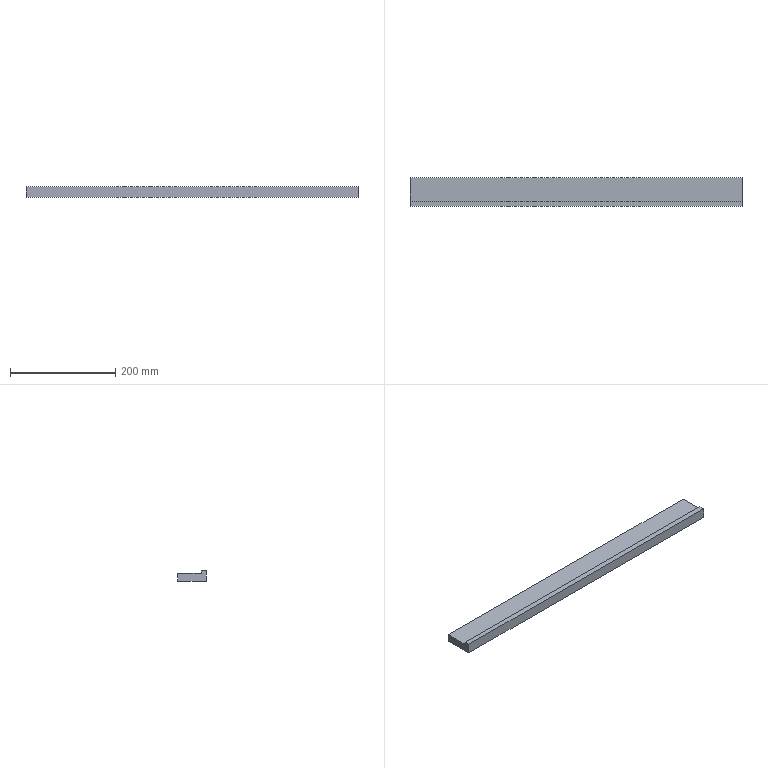Part | SolidWorks | features Extrusion 1 | 1 solid | 8 faces | box 630 x 55 x 20 mm | volume 551250 mm3 | plane 8
STEP:
#1=CARTESIAN_POINT('',(0.,48.109,31.215));
#2=VERTEX_POINT('',#1);
#3=CARTESIAN_POINT('',(0.,48.109,46.215));
#4=VERTEX_POINT('',#3);
#5=CARTESIAN_POINT('',(0.,48.109,31.215));
#6=DIRECTION('',(0.,0.,1.));
#7=VECTOR('',#6,1000.);
#8=LINE('',#5,#7);
#9=EDGE_CURVE('',#2,#4,#8,.T.);
#10=ORIENTED_EDGE('',*,*,#9,.F.);
#11=CARTESIAN_POINT('',(-630.,48.109,31.215));
#12=VERTEX_POINT('',#11);
#13=CARTESIAN_POINT('',(-630.,48.109,31.215));
#14=DIRECTION('',(1.,0.,0.));
#15=VECTOR('',#14,1000.);
#16=LINE('',#13,#15);
#17=EDGE_CURVE('',#12,#2,#16,.T.);
#18=ORIENTED_EDGE('',*,*,#17,.F.);
#19=CARTESIAN_POINT('',(-630.,48.109,46.215));
#20=VERTEX_POINT('',#19);
#21=CARTESIAN_POINT('',(-630.,48.109,31.215));
#22=DIRECTION('',(0.,0.,1.));
#23=VECTOR('',#22,1000.);
#24=LINE('',#21,#23);
#25=EDGE_CURVE('',#12,#20,#24,.T.);
#26=ORIENTED_EDGE('',*,*,#25,.T.);
#27=CARTESIAN_POINT('',(-630.,48.109,46.215));
#28=DIRECTION('',(1.,0.,0.));
#29=VECTOR('',#28,1000.);
#30=LINE('',#27,#29);
#31=EDGE_CURVE('',#20,#4,#30,.T.);
#32=ORIENTED_EDGE('',*,*,#31,.T.);
#33=EDGE_LOOP('',(#10,#18,#26,#32));
#34=FACE_OUTER_BOUND('',#33,.T.);
#35=CARTESIAN_POINT('',(-630.,48.109,31.215));
#36=DIRECTION('',(0.,1.,0.));
#37=DIRECTION('',(0.,0.,1.));
#38=AXIS2_PLACEMENT_3D('',#35,#36,#37);
#39=PLANE('',#38);
#40=ADVANCED_FACE('',(#34),#39,.T.);
#41=CARTESIAN_POINT('',(0.,-6.891,31.215));
#42=VERTEX_POINT('',#41);
#43=CARTESIAN_POINT('',(0.,48.109,31.215));
#44=DIRECTION('',(0.,1.,0.));
#45=VECTOR('',#44,1000.);
#46=LINE('',#43,#45);
#47=EDGE_CURVE('',#42,#2,#46,.T.);
#48=ORIENTED_EDGE('',*,*,#47,.F.);
#49=CARTESIAN_POINT('',(-630.,-6.891,31.215));
#50=VERTEX_POINT('',#49);
#51=CARTESIAN_POINT('',(-630.,-6.891,31.215));
#52=DIRECTION('',(1.,0.,0.));
#53=VECTOR('',#52,1000.);
#54=LINE('',#51,#53);
#55=EDGE_CURVE('',#50,#42,#54,.T.);
#56=ORIENTED_EDGE('',*,*,#55,.F.);
#57=CARTESIAN_POINT('',(-630.,48.109,31.215));
#58=DIRECTION('',(0.,1.,0.));
#59=VECTOR('',#58,1000.);
#60=LINE('',#57,#59);
#61=EDGE_CURVE('',#50,#12,#60,.T.);
#62=ORIENTED_EDGE('',*,*,#61,.T.);
#63=ORIENTED_EDGE('',*,*,#17,.T.);
#64=EDGE_LOOP('',(#48,#56,#62,#63));
#65=FACE_OUTER_BOUND('',#64,.T.);
#66=CARTESIAN_POINT('',(-630.,48.109,31.215));
#67=DIRECTION('',(0.,0.,-1.));
#68=DIRECTION('',(0.,1.,0.));
#69=AXIS2_PLACEMENT_3D('',#66,#67,#68);
#70=PLANE('',#69);
#71=ADVANCED_FACE('',(#65),#70,.T.);
#72=CARTESIAN_POINT('',(0.,-6.891,51.215));
#73=VERTEX_POINT('',#72);
#74=CARTESIAN_POINT('',(0.,-6.891,51.215));
#75=DIRECTION('',(0.,0.,-1.));
#76=VECTOR('',#75,1000.);
#77=LINE('',#74,#76);
#78=EDGE_CURVE('',#73,#42,#77,.T.);
#79=ORIENTED_EDGE('',*,*,#78,.F.);
#80=CARTESIAN_POINT('',(-630.,-6.891,51.215));
#81=VERTEX_POINT('',#80);
#82=CARTESIAN_POINT('',(-630.,-6.891,51.215));
#83=DIRECTION('',(1.,0.,0.));
#84=VECTOR('',#83,1000.);
#85=LINE('',#82,#84);
#86=EDGE_CURVE('',#81,#73,#85,.T.);
#87=ORIENTED_EDGE('',*,*,#86,.F.);
#88=CARTESIAN_POINT('',(-630.,-6.891,51.215));
#89=DIRECTION('',(0.,0.,-1.));
#90=VECTOR('',#89,1000.);
#91=LINE('',#88,#90);
#92=EDGE_CURVE('',#81,#50,#91,.T.);
#93=ORIENTED_EDGE('',*,*,#92,.T.);
#94=ORIENTED_EDGE('',*,*,#55,.T.);
#95=EDGE_LOOP('',(#79,#87,#93,#94));
#96=FACE_OUTER_BOUND('',#95,.T.);
#97=CARTESIAN_POINT('',(-630.,-6.891,51.215));
#98=DIRECTION('',(0.,-1.,0.));
#99=DIRECTION('',(0.,0.,-1.));
#100=AXIS2_PLACEMENT_3D('',#97,#98,#99);
#101=PLANE('',#100);
#102=ADVANCED_FACE('',(#96),#101,.T.);
#103=CARTESIAN_POINT('',(0.,3.109,51.215));
#104=VERTEX_POINT('',#103);
#105=CARTESIAN_POINT('',(0.,-6.891,51.215));
#106=DIRECTION('',(0.,-1.,0.));
#107=VECTOR('',#106,1000.);
#108=LINE('',#105,#107);
#109=EDGE_CURVE('',#104,#73,#108,.T.);
#110=ORIENTED_EDGE('',*,*,#109,.F.);
#111=CARTESIAN_POINT('',(-630.,3.109,51.215));
#112=VERTEX_POINT('',#111);
#113=CARTESIAN_POINT('',(-630.,3.109,51.215));
#114=DIRECTION('',(1.,0.,0.));
#115=VECTOR('',#114,1000.);
#116=LINE('',#113,#115);
#117=EDGE_CURVE('',#112,#104,#116,.T.);
#118=ORIENTED_EDGE('',*,*,#117,.F.);
#119=CARTESIAN_POINT('',(-630.,-6.891,51.215));
#120=DIRECTION('',(0.,-1.,0.));
#121=VECTOR('',#120,1000.);
#122=LINE('',#119,#121);
#123=EDGE_CURVE('',#112,#81,#122,.T.);
#124=ORIENTED_EDGE('',*,*,#123,.T.);
#125=ORIENTED_EDGE('',*,*,#86,.T.);
#126=EDGE_LOOP('',(#110,#118,#124,#125));
#127=FACE_OUTER_BOUND('',#126,.T.);
#128=CARTESIAN_POINT('',(-630.,-6.891,51.215));
#129=DIRECTION('',(0.,0.,1.));
#130=DIRECTION('',(1.,0.,0.));
#131=AXIS2_PLACEMENT_3D('',#128,#129,#130);
#132=PLANE('',#131);
#133=ADVANCED_FACE('',(#127),#132,.T.);
#134=CARTESIAN_POINT('',(0.,3.109,46.215));
#135=VERTEX_POINT('',#134);
#136=CARTESIAN_POINT('',(0.,3.109,51.215));
#137=DIRECTION('',(0.,0.,1.));
#138=VECTOR('',#137,1000.);
#139=LINE('',#136,#138);
#140=EDGE_CURVE('',#135,#104,#139,.T.);
#141=ORIENTED_EDGE('',*,*,#140,.F.);
#142=CARTESIAN_POINT('',(-630.,3.109,46.215));
#143=VERTEX_POINT('',#142);
#144=CARTESIAN_POINT('',(-630.,3.109,46.215));
#145=DIRECTION('',(1.,0.,0.));
#146=VECTOR('',#145,1000.);
#147=LINE('',#144,#146);
#148=EDGE_CURVE('',#143,#135,#147,.T.);
#149=ORIENTED_EDGE('',*,*,#148,.F.);
#150=CARTESIAN_POINT('',(-630.,3.109,51.215));
#151=DIRECTION('',(0.,0.,1.));
#152=VECTOR('',#151,1000.);
#153=LINE('',#150,#152);
#154=EDGE_CURVE('',#143,#112,#153,.T.);
#155=ORIENTED_EDGE('',*,*,#154,.T.);
#156=ORIENTED_EDGE('',*,*,#117,.T.);
#157=EDGE_LOOP('',(#141,#149,#155,#156));
#158=FACE_OUTER_BOUND('',#157,.T.);
#159=CARTESIAN_POINT('',(-630.,3.109,51.215));
#160=DIRECTION('',(0.,1.,0.));
#161=DIRECTION('',(0.,0.,1.));
#162=AXIS2_PLACEMENT_3D('',#159,#160,#161);
#163=PLANE('',#162);
#164=ADVANCED_FACE('',(#158),#163,.T.);
#165=CARTESIAN_POINT('',(0.,48.109,46.215));
#166=DIRECTION('',(0.,-1.,0.));
#167=VECTOR('',#166,1000.);
#168=LINE('',#165,#167);
#169=EDGE_CURVE('',#4,#135,#168,.T.);
#170=ORIENTED_EDGE('',*,*,#169,.F.);
#171=ORIENTED_EDGE('',*,*,#31,.F.);
#172=CARTESIAN_POINT('',(-630.,48.109,46.215));
#173=DIRECTION('',(0.,-1.,0.));
#174=VECTOR('',#173,1000.);
#175=LINE('',#172,#174);
#176=EDGE_CURVE('',#20,#143,#175,.T.);
#177=ORIENTED_EDGE('',*,*,#176,.T.);
#178=ORIENTED_EDGE('',*,*,#148,.T.);
#179=EDGE_LOOP('',(#170,#171,#177,#178));
#180=FACE_OUTER_BOUND('',#179,.T.);
#181=CARTESIAN_POINT('',(-630.,48.109,46.215));
#182=DIRECTION('',(0.,0.,1.));
#183=DIRECTION('',(0.,-1.,0.));
#184=AXIS2_PLACEMENT_3D('',#181,#182,#183);
#185=PLANE('',#184);
#186=ADVANCED_FACE('',(#180),#185,.T.);
#187=ORIENTED_EDGE('',*,*,#25,.F.);
#188=ORIENTED_EDGE('',*,*,#61,.F.);
#189=ORIENTED_EDGE('',*,*,#92,.F.);
#190=ORIENTED_EDGE('',*,*,#123,.F.);
#191=ORIENTED_EDGE('',*,*,#154,.F.);
#192=ORIENTED_EDGE('',*,*,#176,.F.);
#193=EDGE_LOOP('',(#187,#188,#189,#190,#191,#192));
#194=FACE_OUTER_BOUND('',#193,.T.);
#195=CARTESIAN_POINT('',(-630.,0.,0.));
#196=DIRECTION('',(1.,0.,0.));
#197=DIRECTION('',(0.,0.,-1.));
#198=AXIS2_PLACEMENT_3D('',#195,#196,#197);
#199=PLANE('',#198);
#200=ADVANCED_FACE('',(#194),#199,.F.);
#201=ORIENTED_EDGE('',*,*,#9,.T.);
#202=ORIENTED_EDGE('',*,*,#169,.T.);
#203=ORIENTED_EDGE('',*,*,#140,.T.);
#204=ORIENTED_EDGE('',*,*,#109,.T.);
#205=ORIENTED_EDGE('',*,*,#78,.T.);
#206=ORIENTED_EDGE('',*,*,#47,.T.);
#207=EDGE_LOOP('',(#201,#202,#203,#204,#205,#206));
#208=FACE_OUTER_BOUND('',#207,.T.);
#209=CARTESIAN_POINT('',(0.,0.,0.));
#210=DIRECTION('',(1.,0.,0.));
#211=DIRECTION('',(0.,0.,-1.));
#212=AXIS2_PLACEMENT_3D('',#209,#210,#211);
#213=PLANE('',#212);
#214=ADVANCED_FACE('',(#208),#213,.T.);
#215=CLOSED_SHELL('',(#40,#71,#102,#133,#164,#186,#200,#214));
#216=MANIFOLD_SOLID_BREP('',#215);
#217=CARTESIAN_POINT('',(0.,0.,0.));
#218=DIRECTION('',(0.,0.,1.));
#219=DIRECTION('',(1.,0.,0.));
#220=AXIS2_PLACEMENT_3D('',#217,#218,#219);
#221=(LENGTH_UNIT()NAMED_UNIT(*)SI_UNIT(.MILLI.,.METRE.));
#222=UNCERTAINTY_MEASURE_WITH_UNIT(LENGTH_MEASURE(0.00001),#221,'','');
#223=(NAMED_UNIT(*)PLANE_ANGLE_UNIT()SI_UNIT($,.RADIAN.));
#224=(NAMED_UNIT(*)SI_UNIT($,.STERADIAN.)SOLID_ANGLE_UNIT());
#225=(GEOMETRIC_REPRESENTATION_CONTEXT(3)GLOBAL_UNCERTAINTY_ASSIGNED_CONTEXT((#222))GLOBAL_UNIT_ASSIGNED_CONTEXT((#221,#223,#224))REPRESENTATION_CONTEXT('',''));
#226=ADVANCED_BREP_SHAPE_REPRESENTATION('',(#216,#220),#225);